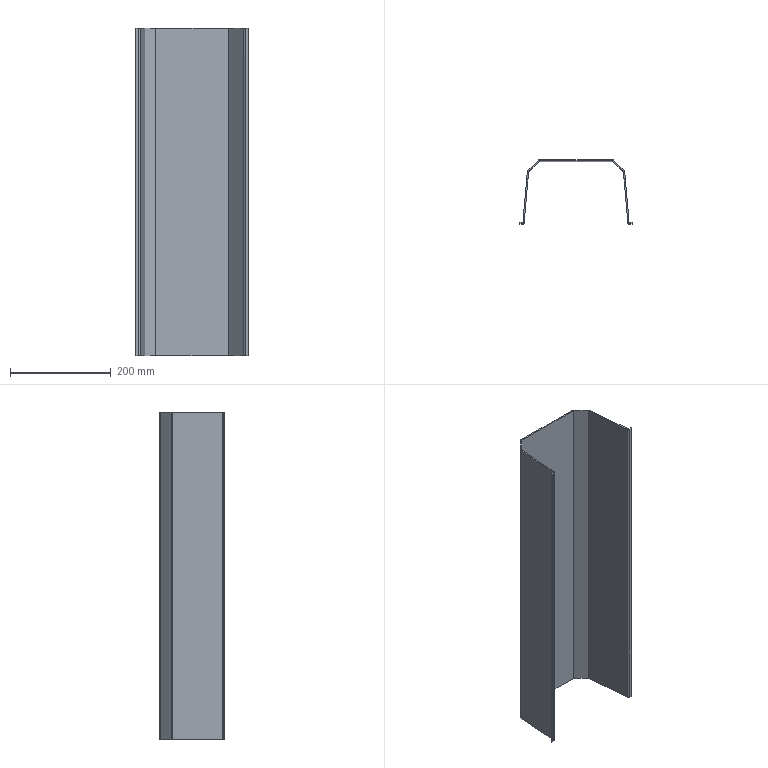Part | STEP file | 51E-01222JG10 | 1 solid | 56 faces | box 225 x 127 x 650 mm | volume 696230 mm3 | plane 40 | cylinder 16 | commonest cylinder face diameters 2 x6 7 x6 2.5 x4
STEP:
#1=CARTESIAN_POINT('',(-106.207,0.,325.));
#2=VERTEX_POINT('',#1);
#3=CARTESIAN_POINT('',(-106.207,2.5,325.));
#4=VERTEX_POINT('',#3);
#5=CARTESIAN_POINT('',(-106.207,1.25,325.));
#6=DIRECTION('',(0.,1.,0.));
#7=VECTOR('',#6,1.);
#8=LINE('',#5,#7);
#9=EDGE_CURVE('',#2,#4,#8,.T.);
#10=ORIENTED_EDGE('',*,*,#9,.F.);
#11=CARTESIAN_POINT('',(-102.72,3.195,325.));
#12=VERTEX_POINT('',#11);
#13=CARTESIAN_POINT('',(-102.72,3.195,325.));
#14=CARTESIAN_POINT('',(-102.752,2.83,325.));
#15=CARTESIAN_POINT('',(-102.832,2.469,325.));
#16=CARTESIAN_POINT('',(-102.959,2.12,325.));
#17=CARTESIAN_POINT('',(-103.301,1.465,325.));
#18=CARTESIAN_POINT('',(-103.8,0.9191,325.));
#19=CARTESIAN_POINT('',(-104.084,0.6808,325.));
#20=CARTESIAN_POINT('',(-104.656,0.3172,325.));
#21=CARTESIAN_POINT('',(-105.296,0.09984,325.));
#22=CARTESIAN_POINT('',(-105.597,0.03328,325.));
#23=CARTESIAN_POINT('',(-105.902,0.,325.));
#24=CARTESIAN_POINT('',(-106.207,0.,325.));
#25=B_SPLINE_CURVE_WITH_KNOTS('',5,(#13,#14,#15,#16,#17,#18,#19,#20,#21,#22,#23,#24),.UNSPECIFIED.,.F.,.U.,(6,3,3,6),(0.,2.592,5.185,7.343),.UNSPECIFIED.);
#26=EDGE_CURVE('',#12,#2,#25,.T.);
#27=ORIENTED_EDGE('',*,*,#26,.F.);
#28=CARTESIAN_POINT('',(-105.211,3.413,325.));
#29=VERTEX_POINT('',#28);
#30=CARTESIAN_POINT('',(-103.966,3.304,325.));
#31=DIRECTION('',(0.9962,-0.08716,0.));
#32=VECTOR('',#31,1.);
#33=LINE('',#30,#32);
#34=EDGE_CURVE('',#29,#12,#33,.T.);
#35=ORIENTED_EDGE('',*,*,#34,.F.);
#36=CARTESIAN_POINT('',(-105.211,3.413,325.));
#37=CARTESIAN_POINT('',(-105.22,3.315,325.));
#38=CARTESIAN_POINT('',(-105.24,3.219,325.));
#39=CARTESIAN_POINT('',(-105.272,3.125,325.));
#40=CARTESIAN_POINT('',(-105.359,2.948,325.));
#41=CARTESIAN_POINT('',(-105.486,2.797,325.));
#42=CARTESIAN_POINT('',(-105.559,2.729,325.));
#43=CARTESIAN_POINT('',(-105.719,2.614,325.));
#44=CARTESIAN_POINT('',(-105.902,2.54,325.));
#45=CARTESIAN_POINT('',(-105.998,2.515,325.));
#46=CARTESIAN_POINT('',(-106.098,2.501,325.));
#47=CARTESIAN_POINT('',(-106.199,2.5,325.));
#48=CARTESIAN_POINT('',(-106.202,2.5,325.));
#49=CARTESIAN_POINT('',(-106.204,2.5,325.));
#50=CARTESIAN_POINT('',(-106.207,2.5,325.));
#51=B_SPLINE_CURVE_WITH_KNOTS('',5,(#36,#37,#38,#39,#40,#41,#42,#43,#44,#45,#46,#47,#48,#49,#50),.UNSPECIFIED.,.F.,.U.,(6,3,3,3,6),(0.,0.6928,1.386,2.078,2.098),.UNSPECIFIED.);
#52=EDGE_CURVE('',#29,#4,#51,.T.);
#53=ORIENTED_EDGE('',*,*,#52,.T.);
#54=EDGE_LOOP('',(#10,#27,#35,#53));
#55=FACE_OUTER_BOUND('',#54,.T.);
#56=CARTESIAN_POINT('',(-106.207,0.,325.));
#57=DIRECTION('',(0.,0.,1.));
#58=DIRECTION('',(1.,0.,0.));
#59=AXIS2_PLACEMENT_3D('',#56,#57,#58);
#60=PLANE('',#59);
#61=ADVANCED_FACE('',(#55),#60,.T.);
#62=CARTESIAN_POINT('',(-111.25,2.5,325.));
#63=VERTEX_POINT('',#62);
#64=CARTESIAN_POINT('',(-112.5,1.25,325.));
#65=VERTEX_POINT('',#64);
#66=CARTESIAN_POINT('',(-111.25,1.25,325.));
#67=DIRECTION('',(0.,0.,1.));
#68=AXIS2_PLACEMENT_3D('',#66,#67,$);
#69=CIRCLE('',#68,1.25);
#70=EDGE_CURVE('',#63,#65,#69,.T.);
#71=ORIENTED_EDGE('',*,*,#70,.T.);
#72=CARTESIAN_POINT('',(-111.25,0.,325.));
#73=VERTEX_POINT('',#72);
#74=CARTESIAN_POINT('',(-111.25,1.25,325.));
#75=DIRECTION('',(0.,0.,1.));
#76=AXIS2_PLACEMENT_3D('',#74,#75,$);
#77=CIRCLE('',#76,1.25);
#78=EDGE_CURVE('',#65,#73,#77,.T.);
#79=ORIENTED_EDGE('',*,*,#78,.T.);
#80=CARTESIAN_POINT('',(-108.729,0.,325.));
#81=DIRECTION('',(-1.,0.,0.));
#82=VECTOR('',#81,1.);
#83=LINE('',#80,#82);
#84=EDGE_CURVE('',#2,#73,#83,.T.);
#85=ORIENTED_EDGE('',*,*,#84,.F.);
#86=ORIENTED_EDGE('',*,*,#9,.T.);
#87=CARTESIAN_POINT('',(-108.729,2.5,325.));
#88=DIRECTION('',(-1.,0.,0.));
#89=VECTOR('',#88,1.);
#90=LINE('',#87,#89);
#91=EDGE_CURVE('',#4,#63,#90,.T.);
#92=ORIENTED_EDGE('',*,*,#91,.T.);
#93=EDGE_LOOP('',(#71,#79,#85,#86,#92));
#94=FACE_OUTER_BOUND('',#93,.T.);
#95=CARTESIAN_POINT('',(-105.211,3.413,325.));
#96=DIRECTION('',(0.,0.,1.));
#97=DIRECTION('',(1.,0.,0.));
#98=AXIS2_PLACEMENT_3D('',#95,#96,#97);
#99=PLANE('',#98);
#100=ADVANCED_FACE('',(#94),#99,.T.);
#101=CARTESIAN_POINT('',(-102.72,3.195,-325.));
#102=VERTEX_POINT('',#101);
#103=CARTESIAN_POINT('',(-106.207,0.,-325.));
#104=VERTEX_POINT('',#103);
#105=CARTESIAN_POINT('',(-106.207,3.5,-325.));
#106=DIRECTION('',(0.,0.,-1.));
#107=AXIS2_PLACEMENT_3D('',#105,#106,$);
#108=CIRCLE('',#107,3.5);
#109=EDGE_CURVE('',#102,#104,#108,.T.);
#110=ORIENTED_EDGE('',*,*,#109,.F.);
#111=CARTESIAN_POINT('',(-102.72,3.195,325.));
#112=DIRECTION('',(0.,0.,-1.));
#113=VECTOR('',#112,1.);
#114=LINE('',#111,#113);
#115=EDGE_CURVE('',#12,#102,#114,.T.);
#116=ORIENTED_EDGE('',*,*,#115,.F.);
#117=ORIENTED_EDGE('',*,*,#26,.T.);
#118=CARTESIAN_POINT('',(-106.207,0.,325.));
#119=DIRECTION('',(0.,0.,-1.));
#120=VECTOR('',#119,1.);
#121=LINE('',#118,#120);
#122=EDGE_CURVE('',#2,#104,#121,.T.);
#123=ORIENTED_EDGE('',*,*,#122,.T.);
#124=EDGE_LOOP('',(#110,#116,#117,#123));
#125=FACE_OUTER_BOUND('',#124,.T.);
#126=CARTESIAN_POINT('',(-106.207,3.5,325.));
#127=DIRECTION('',(0.,0.,-1.));
#128=DIRECTION('',(1.,0.,0.));
#129=AXIS2_PLACEMENT_3D('',#126,#127,#128);
#130=CYLINDRICAL_SURFACE('',#129,3.5);
#131=ADVANCED_FACE('',(#125),#130,.T.);
#132=CARTESIAN_POINT('',(-94.02,102.637,325.));
#133=VERTEX_POINT('',#132);
#134=CARTESIAN_POINT('',(-98.37,52.916,325.));
#135=DIRECTION('',(-0.08716,-0.9962,0.));
#136=VECTOR('',#135,1.);
#137=LINE('',#134,#136);
#138=EDGE_CURVE('',#133,#12,#137,.T.);
#139=ORIENTED_EDGE('',*,*,#138,.F.);
#140=CARTESIAN_POINT('',(-96.511,102.855,325.));
#141=VERTEX_POINT('',#140);
#142=CARTESIAN_POINT('',(-95.266,102.746,325.));
#143=DIRECTION('',(-0.9962,0.08716,0.));
#144=VECTOR('',#143,1.);
#145=LINE('',#142,#144);
#146=EDGE_CURVE('',#133,#141,#145,.T.);
#147=ORIENTED_EDGE('',*,*,#146,.T.);
#148=CARTESIAN_POINT('',(-100.861,53.134,325.));
#149=DIRECTION('',(-0.08716,-0.9962,0.));
#150=VECTOR('',#149,1.);
#151=LINE('',#148,#150);
#152=EDGE_CURVE('',#141,#29,#151,.T.);
#153=ORIENTED_EDGE('',*,*,#152,.T.);
#154=ORIENTED_EDGE('',*,*,#34,.T.);
#155=EDGE_LOOP('',(#139,#147,#153,#154));
#156=FACE_OUTER_BOUND('',#155,.T.);
#157=CARTESIAN_POINT('',(-95.499,105.025,325.));
#158=DIRECTION('',(0.,0.,1.));
#159=DIRECTION('',(1.,0.,0.));
#160=AXIS2_PLACEMENT_3D('',#157,#158,#159);
#161=PLANE('',#160);
#162=ADVANCED_FACE('',(#156),#161,.T.);
#163=CARTESIAN_POINT('',(-105.211,3.413,-325.));
#164=VERTEX_POINT('',#163);
#165=CARTESIAN_POINT('',(-106.207,2.5,-325.));
#166=VERTEX_POINT('',#165);
#167=CARTESIAN_POINT('',(-106.207,3.5,-325.));
#168=DIRECTION('',(0.,0.,-1.));
#169=AXIS2_PLACEMENT_3D('',#167,#168,$);
#170=CIRCLE('',#169,1.);
#171=EDGE_CURVE('',#164,#166,#170,.T.);
#172=ORIENTED_EDGE('',*,*,#171,.T.);
#173=CARTESIAN_POINT('',(-106.207,2.5,325.));
#174=DIRECTION('',(0.,0.,-1.));
#175=VECTOR('',#174,1.);
#176=LINE('',#173,#175);
#177=EDGE_CURVE('',#4,#166,#176,.T.);
#178=ORIENTED_EDGE('',*,*,#177,.F.);
#179=ORIENTED_EDGE('',*,*,#52,.F.);
#180=CARTESIAN_POINT('',(-105.211,3.413,325.));
#181=DIRECTION('',(0.,0.,-1.));
#182=VECTOR('',#181,1.);
#183=LINE('',#180,#182);
#184=EDGE_CURVE('',#29,#164,#183,.T.);
#185=ORIENTED_EDGE('',*,*,#184,.T.);
#186=EDGE_LOOP('',(#172,#178,#179,#185));
#187=FACE_OUTER_BOUND('',#186,.T.);
#188=CARTESIAN_POINT('',(-106.207,3.5,325.));
#189=DIRECTION('',(0.,0.,-1.));
#190=DIRECTION('',(1.,0.,0.));
#191=AXIS2_PLACEMENT_3D('',#188,#189,#190);
#192=CYLINDRICAL_SURFACE('',#191,1.);
#193=ADVANCED_FACE('',(#187),#192,.F.);
#194=CARTESIAN_POINT('',(-112.5,1.25,-325.));
#195=VERTEX_POINT('',#194);
#196=CARTESIAN_POINT('',(-112.5,1.25,325.));
#197=DIRECTION('',(0.,0.,1.));
#198=VECTOR('',#197,1.);
#199=LINE('',#196,#198);
#200=EDGE_CURVE('',#65,#195,#199,.F.);
#201=ORIENTED_EDGE('',*,*,#200,.F.);
#202=ORIENTED_EDGE('',*,*,#70,.F.);
#203=CARTESIAN_POINT('',(-111.25,2.5,-325.));
#204=VERTEX_POINT('',#203);
#205=CARTESIAN_POINT('',(-111.25,2.5,325.));
#206=DIRECTION('',(0.,0.,1.));
#207=VECTOR('',#206,1.);
#208=LINE('',#205,#207);
#209=EDGE_CURVE('',#204,#63,#208,.T.);
#210=ORIENTED_EDGE('',*,*,#209,.F.);
#211=CARTESIAN_POINT('',(-111.25,1.25,-325.));
#212=DIRECTION('',(0.,0.,1.));
#213=AXIS2_PLACEMENT_3D('',#211,#212,$);
#214=CIRCLE('',#213,1.25);
#215=EDGE_CURVE('',#195,#204,#214,.F.);
#216=ORIENTED_EDGE('',*,*,#215,.F.);
#217=EDGE_LOOP('',(#201,#202,#210,#216));
#218=FACE_OUTER_BOUND('',#217,.T.);
#219=CARTESIAN_POINT('',(-111.25,1.25,325.));
#220=DIRECTION('',(0.,0.,1.));
#221=DIRECTION('',(1.,0.,0.));
#222=AXIS2_PLACEMENT_3D('',#219,#220,#221);
#223=CYLINDRICAL_SURFACE('',#222,1.25);
#224=ADVANCED_FACE('',(#218),#223,.T.);
#225=ORIENTED_EDGE('',*,*,#78,.F.);
#226=ORIENTED_EDGE('',*,*,#200,.T.);
#227=CARTESIAN_POINT('',(-111.25,0.,-325.));
#228=VERTEX_POINT('',#227);
#229=CARTESIAN_POINT('',(-111.25,1.25,-325.));
#230=DIRECTION('',(0.,0.,-1.));
#231=AXIS2_PLACEMENT_3D('',#229,#230,$);
#232=CIRCLE('',#231,1.25);
#233=EDGE_CURVE('',#228,#195,#232,.T.);
#234=ORIENTED_EDGE('',*,*,#233,.F.);
#235=CARTESIAN_POINT('',(-111.25,0.,325.));
#236=DIRECTION('',(0.,0.,-1.));
#237=VECTOR('',#236,1.);
#238=LINE('',#235,#237);
#239=EDGE_CURVE('',#73,#228,#238,.T.);
#240=ORIENTED_EDGE('',*,*,#239,.F.);
#241=EDGE_LOOP('',(#225,#226,#234,#240));
#242=FACE_OUTER_BOUND('',#241,.T.);
#243=CARTESIAN_POINT('',(-111.25,1.25,325.));
#244=DIRECTION('',(0.,0.,-1.));
#245=DIRECTION('',(1.,0.,0.));
#246=AXIS2_PLACEMENT_3D('',#243,#244,#245);
#247=CYLINDRICAL_SURFACE('',#246,1.25);
#248=ADVANCED_FACE('',(#242),#247,.T.);
#249=ORIENTED_EDGE('',*,*,#84,.T.);
#250=ORIENTED_EDGE('',*,*,#239,.T.);
#251=CARTESIAN_POINT('',(-108.729,0.,-325.));
#252=DIRECTION('',(-1.,0.,0.));
#253=VECTOR('',#252,1.);
#254=LINE('',#251,#253);
#255=EDGE_CURVE('',#104,#228,#254,.T.);
#256=ORIENTED_EDGE('',*,*,#255,.F.);
#257=ORIENTED_EDGE('',*,*,#122,.F.);
#258=EDGE_LOOP('',(#249,#250,#256,#257));
#259=FACE_OUTER_BOUND('',#258,.T.);
#260=CARTESIAN_POINT('',(-112.5,0.,325.));
#261=DIRECTION('',(0.,-1.,0.));
#262=DIRECTION('',(0.,0.,-1.));
#263=AXIS2_PLACEMENT_3D('',#260,#261,#262);
#264=PLANE('',#263);
#265=ADVANCED_FACE('',(#259),#264,.T.);
#266=CARTESIAN_POINT('',(-108.729,2.5,-325.));
#267=DIRECTION('',(-1.,0.,0.));
#268=VECTOR('',#267,1.);
#269=LINE('',#266,#268);
#270=EDGE_CURVE('',#166,#204,#269,.T.);
#271=ORIENTED_EDGE('',*,*,#270,.T.);
#272=ORIENTED_EDGE('',*,*,#209,.T.);
#273=ORIENTED_EDGE('',*,*,#91,.F.);
#274=ORIENTED_EDGE('',*,*,#177,.T.);
#275=EDGE_LOOP('',(#271,#272,#273,#274));
#276=FACE_OUTER_BOUND('',#275,.T.);
#277=CARTESIAN_POINT('',(-112.5,2.5,325.));
#278=DIRECTION('',(0.,-1.,0.));
#279=DIRECTION('',(0.,0.,-1.));
#280=AXIS2_PLACEMENT_3D('',#277,#278,#279);
#281=PLANE('',#280);
#282=ADVANCED_FACE('',(#276),#281,.F.);
#283=CARTESIAN_POINT('',(-103.966,3.304,-325.));
#284=DIRECTION('',(-0.9962,0.08716,0.));
#285=VECTOR('',#284,1.);
#286=LINE('',#283,#285);
#287=EDGE_CURVE('',#102,#164,#286,.T.);
#288=ORIENTED_EDGE('',*,*,#287,.F.);
#289=ORIENTED_EDGE('',*,*,#109,.T.);
#290=CARTESIAN_POINT('',(-106.207,1.25,-325.));
#291=DIRECTION('',(0.,-1.,0.));
#292=VECTOR('',#291,1.);
#293=LINE('',#290,#292);
#294=EDGE_CURVE('',#166,#104,#293,.T.);
#295=ORIENTED_EDGE('',*,*,#294,.F.);
#296=ORIENTED_EDGE('',*,*,#171,.F.);
#297=EDGE_LOOP('',(#288,#289,#295,#296));
#298=FACE_OUTER_BOUND('',#297,.T.);
#299=CARTESIAN_POINT('',(-102.72,3.195,-325.));
#300=DIRECTION('',(0.,0.,-1.));
#301=DIRECTION('',(-1.,0.,0.));
#302=AXIS2_PLACEMENT_3D('',#299,#300,#301);
#303=PLANE('',#302);
#304=ADVANCED_FACE('',(#298),#303,.T.);
#305=CARTESIAN_POINT('',(-94.02,102.637,-325.));
#306=VERTEX_POINT('',#305);
#307=CARTESIAN_POINT('',(-98.37,52.916,-325.));
#308=DIRECTION('',(-0.08716,-0.9962,0.));
#309=VECTOR('',#308,1.);
#310=LINE('',#307,#309);
#311=EDGE_CURVE('',#306,#102,#310,.T.);
#312=ORIENTED_EDGE('',*,*,#311,.F.);
#313=CARTESIAN_POINT('',(-94.02,102.637,0.));
#314=DIRECTION('',(0.,0.,-1.));
#315=VECTOR('',#314,1.);
#316=LINE('',#313,#315);
#317=EDGE_CURVE('',#133,#306,#316,.T.);
#318=ORIENTED_EDGE('',*,*,#317,.F.);
#319=ORIENTED_EDGE('',*,*,#138,.T.);
#320=ORIENTED_EDGE('',*,*,#115,.T.);
#321=EDGE_LOOP('',(#312,#318,#319,#320));
#322=FACE_OUTER_BOUND('',#321,.T.);
#323=CARTESIAN_POINT('',(-103.,0.,325.));
#324=DIRECTION('',(0.9962,-0.08716,0.));
#325=DIRECTION('',(0.08716,0.9962,0.));
#326=AXIS2_PLACEMENT_3D('',#323,#324,#325);
#327=PLANE('',#326);
#328=ADVANCED_FACE('',(#322),#327,.T.);
#329=ORIENTED_EDGE('',*,*,#146,.F.);
#330=CARTESIAN_POINT('',(-93.731,103.257,325.));
#331=VERTEX_POINT('',#330);
#332=CARTESIAN_POINT('',(-93.024,102.55,325.));
#333=DIRECTION('',(0.,0.,1.));
#334=AXIS2_PLACEMENT_3D('',#332,#333,$);
#335=CIRCLE('',#334,1.);
#336=EDGE_CURVE('',#331,#133,#335,.T.);
#337=ORIENTED_EDGE('',*,*,#336,.F.);
#338=CARTESIAN_POINT('',(-95.499,105.025,325.));
#339=VERTEX_POINT('',#338);
#340=CARTESIAN_POINT('',(-94.615,104.141,325.));
#341=DIRECTION('',(0.7071,-0.7071,0.));
#342=VECTOR('',#341,1.);
#343=LINE('',#340,#342);
#344=EDGE_CURVE('',#339,#331,#343,.T.);
#345=ORIENTED_EDGE('',*,*,#344,.F.);
#346=CARTESIAN_POINT('',(-93.024,102.55,325.));
#347=DIRECTION('',(0.,0.,1.));
#348=AXIS2_PLACEMENT_3D('',#346,#347,$);
#349=CIRCLE('',#348,3.5);
#350=EDGE_CURVE('',#339,#141,#349,.T.);
#351=ORIENTED_EDGE('',*,*,#350,.T.);
#352=EDGE_LOOP('',(#329,#337,#345,#351));
#353=FACE_OUTER_BOUND('',#352,.T.);
#354=CARTESIAN_POINT('',(-94.02,102.637,325.));
#355=DIRECTION('',(0.,0.,1.));
#356=DIRECTION('',(1.,0.,0.));
#357=AXIS2_PLACEMENT_3D('',#354,#355,#356);
#358=PLANE('',#357);
#359=ADVANCED_FACE('',(#353),#358,.T.);
#360=CARTESIAN_POINT('',(-96.511,102.855,-325.));
#361=VERTEX_POINT('',#360);
#362=CARTESIAN_POINT('',(-100.861,53.134,-325.));
#363=DIRECTION('',(-0.08716,-0.9962,0.));
#364=VECTOR('',#363,1.);
#365=LINE('',#362,#364);
#366=EDGE_CURVE('',#361,#164,#365,.T.);
#367=ORIENTED_EDGE('',*,*,#366,.T.);
#368=ORIENTED_EDGE('',*,*,#184,.F.);
#369=ORIENTED_EDGE('',*,*,#152,.F.);
#370=CARTESIAN_POINT('',(-96.511,102.855,0.));
#371=DIRECTION('',(0.,0.,-1.));
#372=VECTOR('',#371,1.);
#373=LINE('',#370,#372);
#374=EDGE_CURVE('',#141,#361,#373,.T.);
#375=ORIENTED_EDGE('',*,*,#374,.T.);
#376=EDGE_LOOP('',(#367,#368,#369,#375));
#377=FACE_OUTER_BOUND('',#376,.T.);
#378=CARTESIAN_POINT('',(-105.49,0.2179,325.));
#379=DIRECTION('',(0.9962,-0.08716,0.));
#380=DIRECTION('',(0.08716,0.9962,0.));
#381=AXIS2_PLACEMENT_3D('',#378,#379,#380);
#382=PLANE('',#381);
#383=ADVANCED_FACE('',(#377),#382,.F.);
#384=ORIENTED_EDGE('',*,*,#255,.T.);
#385=ORIENTED_EDGE('',*,*,#233,.T.);
#386=ORIENTED_EDGE('',*,*,#215,.T.);
#387=ORIENTED_EDGE('',*,*,#270,.F.);
#388=ORIENTED_EDGE('',*,*,#294,.T.);
#389=EDGE_LOOP('',(#384,#385,#386,#387,#388));
#390=FACE_OUTER_BOUND('',#389,.T.);
#391=CARTESIAN_POINT('',(-106.207,3.5,-325.));
#392=DIRECTION('',(0.,0.,-1.));
#393=DIRECTION('',(-1.,0.,0.));
#394=AXIS2_PLACEMENT_3D('',#391,#392,#393);
#395=PLANE('',#394);
#396=ADVANCED_FACE('',(#390),#395,.T.);
#397=ORIENTED_EDGE('',*,*,#311,.T.);
#398=ORIENTED_EDGE('',*,*,#287,.T.);
#399=ORIENTED_EDGE('',*,*,#366,.F.);
#400=CARTESIAN_POINT('',(-95.266,102.746,-325.));
#401=DIRECTION('',(0.9962,-0.08716,0.));
#402=VECTOR('',#401,1.);
#403=LINE('',#400,#402);
#404=EDGE_CURVE('',#361,#306,#403,.T.);
#405=ORIENTED_EDGE('',*,*,#404,.T.);
#406=EDGE_LOOP('',(#397,#398,#399,#405));
#407=FACE_OUTER_BOUND('',#406,.T.);
#408=CARTESIAN_POINT('',(-106.207,2.5,-325.));
#409=DIRECTION('',(0.,0.,-1.));
#410=DIRECTION('',(-1.,0.,0.));
#411=AXIS2_PLACEMENT_3D('',#408,#409,#410);
#412=PLANE('',#411);
#413=ADVANCED_FACE('',(#407),#412,.T.);
#414=CARTESIAN_POINT('',(-93.731,103.257,-325.));
#415=VERTEX_POINT('',#414);
#416=CARTESIAN_POINT('',(-93.024,102.55,-325.));
#417=DIRECTION('',(0.,0.,-1.));
#418=AXIS2_PLACEMENT_3D('',#416,#417,$);
#419=CIRCLE('',#418,1.);
#420=EDGE_CURVE('',#415,#306,#419,.F.);
#421=ORIENTED_EDGE('',*,*,#420,.F.);
#422=CARTESIAN_POINT('',(-93.731,103.257,325.));
#423=DIRECTION('',(0.,0.,-1.));
#424=VECTOR('',#423,1.);
#425=LINE('',#422,#424);
#426=EDGE_CURVE('',#331,#415,#425,.T.);
#427=ORIENTED_EDGE('',*,*,#426,.F.);
#428=ORIENTED_EDGE('',*,*,#336,.T.);
#429=ORIENTED_EDGE('',*,*,#317,.T.);
#430=EDGE_LOOP('',(#421,#427,#428,#429));
#431=FACE_OUTER_BOUND('',#430,.T.);
#432=CARTESIAN_POINT('',(-93.024,102.55,325.));
#433=DIRECTION('',(0.,0.,-1.));
#434=DIRECTION('',(-1.,0.,0.));
#435=AXIS2_PLACEMENT_3D('',#432,#433,#434);
#436=CYLINDRICAL_SURFACE('',#435,1.);
#437=ADVANCED_FACE('',(#431),#436,.F.);
#438=CARTESIAN_POINT('',(-72.782,124.207,325.));
#439=VERTEX_POINT('',#438);
#440=CARTESIAN_POINT('',(-83.256,113.732,325.));
#441=DIRECTION('',(-0.7071,-0.7071,0.));
#442=VECTOR('',#441,1.);
#443=LINE('',#440,#442);
#444=EDGE_CURVE('',#439,#331,#443,.T.);
#445=ORIENTED_EDGE('',*,*,#444,.F.);
#446=CARTESIAN_POINT('',(-74.549,125.975,325.));
#447=VERTEX_POINT('',#446);
#448=CARTESIAN_POINT('',(-73.665,125.091,325.));
#449=DIRECTION('',(-0.7071,0.7071,0.));
#450=VECTOR('',#449,1.);
#451=LINE('',#448,#450);
#452=EDGE_CURVE('',#439,#447,#451,.T.);
#453=ORIENTED_EDGE('',*,*,#452,.T.);
#454=CARTESIAN_POINT('',(-85.024,115.5,325.));
#455=DIRECTION('',(-0.7071,-0.7071,0.));
#456=VECTOR('',#455,1.);
#457=LINE('',#454,#456);
#458=EDGE_CURVE('',#447,#339,#457,.T.);
#459=ORIENTED_EDGE('',*,*,#458,.T.);
#460=ORIENTED_EDGE('',*,*,#344,.T.);
#461=EDGE_LOOP('',(#445,#453,#459,#460));
#462=FACE_OUTER_BOUND('',#461,.T.);
#463=CARTESIAN_POINT('',(-72.074,127.,325.));
#464=DIRECTION('',(0.,0.,1.));
#465=DIRECTION('',(1.,0.,0.));
#466=AXIS2_PLACEMENT_3D('',#463,#464,#465);
#467=PLANE('',#466);
#468=ADVANCED_FACE('',(#462),#467,.T.);
#469=CARTESIAN_POINT('',(-95.499,105.025,-325.));
#470=VERTEX_POINT('',#469);
#471=CARTESIAN_POINT('',(-93.024,102.55,-325.));
#472=DIRECTION('',(0.,0.,-1.));
#473=AXIS2_PLACEMENT_3D('',#471,#472,$);
#474=CIRCLE('',#473,3.5);
#475=EDGE_CURVE('',#470,#361,#474,.F.);
#476=ORIENTED_EDGE('',*,*,#475,.T.);
#477=ORIENTED_EDGE('',*,*,#374,.F.);
#478=ORIENTED_EDGE('',*,*,#350,.F.);
#479=CARTESIAN_POINT('',(-95.499,105.025,325.));
#480=DIRECTION('',(0.,0.,-1.));
#481=VECTOR('',#480,1.);
#482=LINE('',#479,#481);
#483=EDGE_CURVE('',#339,#470,#482,.T.);
#484=ORIENTED_EDGE('',*,*,#483,.T.);
#485=EDGE_LOOP('',(#476,#477,#478,#484));
#486=FACE_OUTER_BOUND('',#485,.T.);
#487=CARTESIAN_POINT('',(-93.024,102.55,325.));
#488=DIRECTION('',(0.,0.,-1.));
#489=DIRECTION('',(-1.,0.,0.));
#490=AXIS2_PLACEMENT_3D('',#487,#488,#489);
#491=CYLINDRICAL_SURFACE('',#490,3.5);
#492=ADVANCED_FACE('',(#486),#491,.T.);
#493=CARTESIAN_POINT('',(-94.615,104.141,-325.));
#494=DIRECTION('',(-0.7071,0.7071,0.));
#495=VECTOR('',#494,1.);
#496=LINE('',#493,#495);
#497=EDGE_CURVE('',#415,#470,#496,.T.);
#498=ORIENTED_EDGE('',*,*,#497,.F.);
#499=ORIENTED_EDGE('',*,*,#420,.T.);
#500=ORIENTED_EDGE('',*,*,#404,.F.);
#501=ORIENTED_EDGE('',*,*,#475,.F.);
#502=EDGE_LOOP('',(#498,#499,#500,#501));
#503=FACE_OUTER_BOUND('',#502,.T.);
#504=CARTESIAN_POINT('',(-93.731,103.257,-325.));
#505=DIRECTION('',(0.,0.,-1.));
#506=DIRECTION('',(-1.,0.,0.));
#507=AXIS2_PLACEMENT_3D('',#504,#505,#506);
#508=PLANE('',#507);
#509=ADVANCED_FACE('',(#503),#508,.T.);
#510=CARTESIAN_POINT('',(-72.782,124.207,-325.));
#511=VERTEX_POINT('',#510);
#512=CARTESIAN_POINT('',(-83.256,113.732,-325.));
#513=DIRECTION('',(-0.7071,-0.7071,0.));
#514=VECTOR('',#513,1.);
#515=LINE('',#512,#514);
#516=EDGE_CURVE('',#511,#415,#515,.T.);
#517=ORIENTED_EDGE('',*,*,#516,.F.);
#518=CARTESIAN_POINT('',(-72.782,124.207,0.));
#519=DIRECTION('',(0.,0.,-1.));
#520=VECTOR('',#519,1.);
#521=LINE('',#518,#520);
#522=EDGE_CURVE('',#439,#511,#521,.T.);
#523=ORIENTED_EDGE('',*,*,#522,.F.);
#524=ORIENTED_EDGE('',*,*,#444,.T.);
#525=ORIENTED_EDGE('',*,*,#426,.T.);
#526=EDGE_LOOP('',(#517,#523,#524,#525));
#527=FACE_OUTER_BOUND('',#526,.T.);
#528=CARTESIAN_POINT('',(-93.989,103.,325.));
#529=DIRECTION('',(0.7071,-0.7071,0.));
#530=DIRECTION('',(0.7071,0.7071,0.));
#531=AXIS2_PLACEMENT_3D('',#528,#529,#530);
#532=PLANE('',#531);
#533=ADVANCED_FACE('',(#527),#532,.T.);
#534=ORIENTED_EDGE('',*,*,#452,.F.);
#535=CARTESIAN_POINT('',(-72.074,124.5,325.));
#536=VERTEX_POINT('',#535);
#537=CARTESIAN_POINT('',(-72.074,123.5,325.));
#538=DIRECTION('',(0.,0.,1.));
#539=AXIS2_PLACEMENT_3D('',#537,#538,$);
#540=CIRCLE('',#539,1.);
#541=EDGE_CURVE('',#536,#439,#540,.T.);
#542=ORIENTED_EDGE('',*,*,#541,.F.);
#543=CARTESIAN_POINT('',(-72.074,127.,325.));
#544=VERTEX_POINT('',#543);
#545=CARTESIAN_POINT('',(-72.074,125.75,325.));
#546=DIRECTION('',(0.,-1.,0.));
#547=VECTOR('',#546,1.);
#548=LINE('',#545,#547);
#549=EDGE_CURVE('',#544,#536,#548,.T.);
#550=ORIENTED_EDGE('',*,*,#549,.F.);
#551=CARTESIAN_POINT('',(-72.074,123.5,325.));
#552=DIRECTION('',(0.,0.,1.));
#553=AXIS2_PLACEMENT_3D('',#551,#552,$);
#554=CIRCLE('',#553,3.5);
#555=EDGE_CURVE('',#544,#447,#554,.T.);
#556=ORIENTED_EDGE('',*,*,#555,.T.);
#557=EDGE_LOOP('',(#534,#542,#550,#556));
#558=FACE_OUTER_BOUND('',#557,.T.);
#559=CARTESIAN_POINT('',(-72.782,124.207,325.));
#560=DIRECTION('',(0.,0.,1.));
#561=DIRECTION('',(1.,0.,0.));
#562=AXIS2_PLACEMENT_3D('',#559,#560,#561);
#563=PLANE('',#562);
#564=ADVANCED_FACE('',(#558),#563,.T.);
#565=CARTESIAN_POINT('',(-74.549,125.975,-325.));
#566=VERTEX_POINT('',#565);
#567=CARTESIAN_POINT('',(-85.024,115.5,-325.));
#568=DIRECTION('',(-0.7071,-0.7071,0.));
#569=VECTOR('',#568,1.);
#570=LINE('',#567,#569);
#571=EDGE_CURVE('',#566,#470,#570,.T.);
#572=ORIENTED_EDGE('',*,*,#571,.T.);
#573=ORIENTED_EDGE('',*,*,#483,.F.);
#574=ORIENTED_EDGE('',*,*,#458,.F.);
#575=CARTESIAN_POINT('',(-74.549,125.975,0.));
#576=DIRECTION('',(0.,0.,-1.));
#577=VECTOR('',#576,1.);
#578=LINE('',#575,#577);
#579=EDGE_CURVE('',#447,#566,#578,.T.);
#580=ORIENTED_EDGE('',*,*,#579,.T.);
#581=EDGE_LOOP('',(#572,#573,#574,#580));
#582=FACE_OUTER_BOUND('',#581,.T.);
#583=CARTESIAN_POINT('',(-95.756,104.768,325.));
#584=DIRECTION('',(0.7071,-0.7071,0.));
#585=DIRECTION('',(0.7071,0.7071,0.));
#586=AXIS2_PLACEMENT_3D('',#583,#584,#585);
#587=PLANE('',#586);
#588=ADVANCED_FACE('',(#582),#587,.F.);
#589=ORIENTED_EDGE('',*,*,#516,.T.);
#590=ORIENTED_EDGE('',*,*,#497,.T.);
#591=ORIENTED_EDGE('',*,*,#571,.F.);
#592=CARTESIAN_POINT('',(-73.665,125.091,-325.));
#593=DIRECTION('',(0.7071,-0.7071,0.));
#594=VECTOR('',#593,1.);
#595=LINE('',#592,#594);
#596=EDGE_CURVE('',#566,#511,#595,.T.);
#597=ORIENTED_EDGE('',*,*,#596,.T.);
#598=EDGE_LOOP('',(#589,#590,#591,#597));
#599=FACE_OUTER_BOUND('',#598,.T.);
#600=CARTESIAN_POINT('',(-96.511,102.855,-325.));
#601=DIRECTION('',(0.,0.,-1.));
#602=DIRECTION('',(-1.,0.,0.));
#603=AXIS2_PLACEMENT_3D('',#600,#601,#602);
#604=PLANE('',#603);
#605=ADVANCED_FACE('',(#599),#604,.T.);
#606=CARTESIAN_POINT('',(-72.074,124.5,-325.));
#607=VERTEX_POINT('',#606);
#608=CARTESIAN_POINT('',(-72.074,123.5,-325.));
#609=DIRECTION('',(0.,0.,-1.));
#610=AXIS2_PLACEMENT_3D('',#608,#609,$);
#611=CIRCLE('',#610,1.);
#612=EDGE_CURVE('',#607,#511,#611,.F.);
#613=ORIENTED_EDGE('',*,*,#612,.F.);
#614=CARTESIAN_POINT('',(-72.074,124.5,325.));
#615=DIRECTION('',(0.,0.,-1.));
#616=VECTOR('',#615,1.);
#617=LINE('',#614,#616);
#618=EDGE_CURVE('',#536,#607,#617,.T.);
#619=ORIENTED_EDGE('',*,*,#618,.F.);
#620=ORIENTED_EDGE('',*,*,#541,.T.);
#621=ORIENTED_EDGE('',*,*,#522,.T.);
#622=EDGE_LOOP('',(#613,#619,#620,#621));
#623=FACE_OUTER_BOUND('',#622,.T.);
#624=CARTESIAN_POINT('',(-72.074,123.5,325.));
#625=DIRECTION('',(0.,0.,-1.));
#626=DIRECTION('',(-1.,0.,0.));
#627=AXIS2_PLACEMENT_3D('',#624,#625,#626);
#628=CYLINDRICAL_SURFACE('',#627,1.);
#629=ADVANCED_FACE('',(#623),#628,.F.);
#630=CARTESIAN_POINT('',(72.074,124.5,325.));
#631=VERTEX_POINT('',#630);
#632=CARTESIAN_POINT('',(0.,124.5,325.));
#633=DIRECTION('',(-1.,0.,0.));
#634=VECTOR('',#633,1.);
#635=LINE('',#632,#634);
#636=EDGE_CURVE('',#631,#536,#635,.T.);
#637=ORIENTED_EDGE('',*,*,#636,.F.);
#638=CARTESIAN_POINT('',(72.074,127.,325.));
#639=VERTEX_POINT('',#638);
#640=CARTESIAN_POINT('',(72.074,125.75,325.));
#641=DIRECTION('',(0.,1.,0.));
#642=VECTOR('',#641,1.);
#643=LINE('',#640,#642);
#644=EDGE_CURVE('',#631,#639,#643,.T.);
#645=ORIENTED_EDGE('',*,*,#644,.T.);
#646=CARTESIAN_POINT('',(0.,127.,325.));
#647=DIRECTION('',(-1.,0.,0.));
#648=VECTOR('',#647,1.);
#649=LINE('',#646,#648);
#650=EDGE_CURVE('',#639,#544,#649,.T.);
#651=ORIENTED_EDGE('',*,*,#650,.T.);
#652=ORIENTED_EDGE('',*,*,#549,.T.);
#653=EDGE_LOOP('',(#637,#645,#651,#652));
#654=FACE_OUTER_BOUND('',#653,.T.);
#655=CARTESIAN_POINT('',(74.549,125.975,325.));
#656=DIRECTION('',(0.,0.,1.));
#657=DIRECTION('',(1.,0.,0.));
#658=AXIS2_PLACEMENT_3D('',#655,#656,#657);
#659=PLANE('',#658);
#660=ADVANCED_FACE('',(#654),#659,.T.);
#661=CARTESIAN_POINT('',(-72.074,127.,-325.));
#662=VERTEX_POINT('',#661);
#663=CARTESIAN_POINT('',(-72.074,123.5,-325.));
#664=DIRECTION('',(0.,0.,-1.));
#665=AXIS2_PLACEMENT_3D('',#663,#664,$);
#666=CIRCLE('',#665,3.5);
#667=EDGE_CURVE('',#662,#566,#666,.F.);
#668=ORIENTED_EDGE('',*,*,#667,.T.);
#669=ORIENTED_EDGE('',*,*,#579,.F.);
#670=ORIENTED_EDGE('',*,*,#555,.F.);
#671=CARTESIAN_POINT('',(-72.074,127.,325.));
#672=DIRECTION('',(0.,0.,-1.));
#673=VECTOR('',#672,1.);
#674=LINE('',#671,#673);
#675=EDGE_CURVE('',#544,#662,#674,.T.);
#676=ORIENTED_EDGE('',*,*,#675,.T.);
#677=EDGE_LOOP('',(#668,#669,#670,#676));
#678=FACE_OUTER_BOUND('',#677,.T.);
#679=CARTESIAN_POINT('',(-72.074,123.5,325.));
#680=DIRECTION('',(0.,0.,-1.));
#681=DIRECTION('',(-1.,0.,0.));
#682=AXIS2_PLACEMENT_3D('',#679,#680,#681);
#683=CYLINDRICAL_SURFACE('',#682,3.5);
#684=ADVANCED_FACE('',(#678),#683,.T.);
#685=CARTESIAN_POINT('',(-72.074,125.75,-325.));
#686=DIRECTION('',(0.,1.,0.));
#687=VECTOR('',#686,1.);
#688=LINE('',#685,#687);
#689=EDGE_CURVE('',#607,#662,#688,.T.);
#690=ORIENTED_EDGE('',*,*,#689,.F.);
#691=ORIENTED_EDGE('',*,*,#612,.T.);
#692=ORIENTED_EDGE('',*,*,#596,.F.);
#693=ORIENTED_EDGE('',*,*,#667,.F.);
#694=EDGE_LOOP('',(#690,#691,#692,#693));
#695=FACE_OUTER_BOUND('',#694,.T.);
#696=CARTESIAN_POINT('',(-72.074,124.5,-325.));
#697=DIRECTION('',(0.,0.,-1.));
#698=DIRECTION('',(-1.,0.,0.));
#699=AXIS2_PLACEMENT_3D('',#696,#697,#698);
#700=PLANE('',#699);
#701=ADVANCED_FACE('',(#695),#700,.T.);
#702=CARTESIAN_POINT('',(72.074,124.5,-325.));
#703=VERTEX_POINT('',#702);
#704=CARTESIAN_POINT('',(0.,124.5,-325.));
#705=DIRECTION('',(-1.,0.,0.));
#706=VECTOR('',#705,1.);
#707=LINE('',#704,#706);
#708=EDGE_CURVE('',#703,#607,#707,.T.);
#709=ORIENTED_EDGE('',*,*,#708,.F.);
#710=CARTESIAN_POINT('',(72.074,124.5,0.));
#711=DIRECTION('',(0.,0.,-1.));
#712=VECTOR('',#711,1.);
#713=LINE('',#710,#712);
#714=EDGE_CURVE('',#631,#703,#713,.T.);
#715=ORIENTED_EDGE('',*,*,#714,.F.);
#716=ORIENTED_EDGE('',*,*,#636,.T.);
#717=ORIENTED_EDGE('',*,*,#618,.T.);
#718=EDGE_LOOP('',(#709,#715,#716,#717));
#719=FACE_OUTER_BOUND('',#718,.T.);
#720=CARTESIAN_POINT('',(-72.489,124.5,325.));
#721=DIRECTION('',(0.,-1.,0.));
#722=DIRECTION('',(0.,0.,-1.));
#723=AXIS2_PLACEMENT_3D('',#720,#721,#722);
#724=PLANE('',#723);
#725=ADVANCED_FACE('',(#719),#724,.T.);
#726=ORIENTED_EDGE('',*,*,#644,.F.);
#727=CARTESIAN_POINT('',(72.782,124.207,325.));
#728=VERTEX_POINT('',#727);
#729=CARTESIAN_POINT('',(72.074,123.5,325.));
#730=DIRECTION('',(0.,0.,1.));
#731=AXIS2_PLACEMENT_3D('',#729,#730,$);
#732=CIRCLE('',#731,1.);
#733=EDGE_CURVE('',#728,#631,#732,.T.);
#734=ORIENTED_EDGE('',*,*,#733,.F.);
#735=CARTESIAN_POINT('',(74.549,125.975,325.));
#736=VERTEX_POINT('',#735);
#737=CARTESIAN_POINT('',(73.665,125.091,325.));
#738=DIRECTION('',(-0.7071,-0.7071,0.));
#739=VECTOR('',#738,1.);
#740=LINE('',#737,#739);
#741=EDGE_CURVE('',#736,#728,#740,.T.);
#742=ORIENTED_EDGE('',*,*,#741,.F.);
#743=CARTESIAN_POINT('',(72.074,123.5,325.));
#744=DIRECTION('',(0.,0.,1.));
#745=AXIS2_PLACEMENT_3D('',#743,#744,$);
#746=CIRCLE('',#745,3.5);
#747=EDGE_CURVE('',#736,#639,#746,.T.);
#748=ORIENTED_EDGE('',*,*,#747,.T.);
#749=EDGE_LOOP('',(#726,#734,#742,#748));
#750=FACE_OUTER_BOUND('',#749,.T.);
#751=CARTESIAN_POINT('',(72.074,124.5,325.));
#752=DIRECTION('',(0.,0.,1.));
#753=DIRECTION('',(1.,0.,0.));
#754=AXIS2_PLACEMENT_3D('',#751,#752,#753);
#755=PLANE('',#754);
#756=ADVANCED_FACE('',(#750),#755,.T.);
#757=CARTESIAN_POINT('',(72.074,127.,-325.));
#758=VERTEX_POINT('',#757);
#759=CARTESIAN_POINT('',(0.,127.,-325.));
#760=DIRECTION('',(-1.,0.,0.));
#761=VECTOR('',#760,1.);
#762=LINE('',#759,#761);
#763=EDGE_CURVE('',#758,#662,#762,.T.);
#764=ORIENTED_EDGE('',*,*,#763,.T.);
#765=ORIENTED_EDGE('',*,*,#675,.F.);
#766=ORIENTED_EDGE('',*,*,#650,.F.);
#767=CARTESIAN_POINT('',(72.074,127.,0.));
#768=DIRECTION('',(0.,0.,-1.));
#769=VECTOR('',#768,1.);
#770=LINE('',#767,#769);
#771=EDGE_CURVE('',#639,#758,#770,.T.);
#772=ORIENTED_EDGE('',*,*,#771,.T.);
#773=EDGE_LOOP('',(#764,#765,#766,#772));
#774=FACE_OUTER_BOUND('',#773,.T.);
#775=CARTESIAN_POINT('',(-72.489,127.,325.));
#776=DIRECTION('',(0.,-1.,0.));
#777=DIRECTION('',(0.,0.,-1.));
#778=AXIS2_PLACEMENT_3D('',#775,#776,#777);
#779=PLANE('',#778);
#780=ADVANCED_FACE('',(#774),#779,.F.);
#781=ORIENTED_EDGE('',*,*,#708,.T.);
#782=ORIENTED_EDGE('',*,*,#689,.T.);
#783=ORIENTED_EDGE('',*,*,#763,.F.);
#784=CARTESIAN_POINT('',(72.074,125.75,-325.));
#785=DIRECTION('',(0.,-1.,0.));
#786=VECTOR('',#785,1.);
#787=LINE('',#784,#786);
#788=EDGE_CURVE('',#758,#703,#787,.T.);
#789=ORIENTED_EDGE('',*,*,#788,.T.);
#790=EDGE_LOOP('',(#781,#782,#783,#789));
#791=FACE_OUTER_BOUND('',#790,.T.);
#792=CARTESIAN_POINT('',(-74.549,125.975,-325.));
#793=DIRECTION('',(0.,0.,-1.));
#794=DIRECTION('',(-1.,0.,0.));
#795=AXIS2_PLACEMENT_3D('',#792,#793,#794);
#796=PLANE('',#795);
#797=ADVANCED_FACE('',(#791),#796,.T.);
#798=CARTESIAN_POINT('',(72.782,124.207,-325.));
#799=VERTEX_POINT('',#798);
#800=CARTESIAN_POINT('',(72.074,123.5,-325.));
#801=DIRECTION('',(0.,0.,-1.));
#802=AXIS2_PLACEMENT_3D('',#800,#801,$);
#803=CIRCLE('',#802,1.);
#804=EDGE_CURVE('',#799,#703,#803,.F.);
#805=ORIENTED_EDGE('',*,*,#804,.F.);
#806=CARTESIAN_POINT('',(72.782,124.207,325.));
#807=DIRECTION('',(0.,0.,-1.));
#808=VECTOR('',#807,1.);
#809=LINE('',#806,#808);
#810=EDGE_CURVE('',#728,#799,#809,.T.);
#811=ORIENTED_EDGE('',*,*,#810,.F.);
#812=ORIENTED_EDGE('',*,*,#733,.T.);
#813=ORIENTED_EDGE('',*,*,#714,.T.);
#814=EDGE_LOOP('',(#805,#811,#812,#813));
#815=FACE_OUTER_BOUND('',#814,.T.);
#816=CARTESIAN_POINT('',(72.074,123.5,325.));
#817=DIRECTION('',(0.,0.,-1.));
#818=DIRECTION('',(-1.,0.,0.));
#819=AXIS2_PLACEMENT_3D('',#816,#817,#818);
#820=CYLINDRICAL_SURFACE('',#819,1.);
#821=ADVANCED_FACE('',(#815),#820,.F.);
#822=CARTESIAN_POINT('',(93.731,103.257,325.));
#823=VERTEX_POINT('',#822);
#824=CARTESIAN_POINT('',(83.256,113.732,325.));
#825=DIRECTION('',(-0.7071,0.7071,0.));
#826=VECTOR('',#825,1.);
#827=LINE('',#824,#826);
#828=EDGE_CURVE('',#823,#728,#827,.T.);
#829=ORIENTED_EDGE('',*,*,#828,.F.);
#830=CARTESIAN_POINT('',(95.499,105.025,325.));
#831=VERTEX_POINT('',#830);
#832=CARTESIAN_POINT('',(94.615,104.141,325.));
#833=DIRECTION('',(0.7071,0.7071,0.));
#834=VECTOR('',#833,1.);
#835=LINE('',#832,#834);
#836=EDGE_CURVE('',#823,#831,#835,.T.);
#837=ORIENTED_EDGE('',*,*,#836,.T.);
#838=CARTESIAN_POINT('',(85.024,115.5,325.));
#839=DIRECTION('',(-0.7071,0.7071,0.));
#840=VECTOR('',#839,1.);
#841=LINE('',#838,#840);
#842=EDGE_CURVE('',#831,#736,#841,.T.);
#843=ORIENTED_EDGE('',*,*,#842,.T.);
#844=ORIENTED_EDGE('',*,*,#741,.T.);
#845=EDGE_LOOP('',(#829,#837,#843,#844));
#846=FACE_OUTER_BOUND('',#845,.T.);
#847=CARTESIAN_POINT('',(96.511,102.855,325.));
#848=DIRECTION('',(0.,0.,1.));
#849=DIRECTION('',(1.,0.,0.));
#850=AXIS2_PLACEMENT_3D('',#847,#848,#849);
#851=PLANE('',#850);
#852=ADVANCED_FACE('',(#846),#851,.T.);
#853=CARTESIAN_POINT('',(74.549,125.975,-325.));
#854=VERTEX_POINT('',#853);
#855=CARTESIAN_POINT('',(72.074,123.5,-325.));
#856=DIRECTION('',(0.,0.,-1.));
#857=AXIS2_PLACEMENT_3D('',#855,#856,$);
#858=CIRCLE('',#857,3.5);
#859=EDGE_CURVE('',#854,#758,#858,.F.);
#860=ORIENTED_EDGE('',*,*,#859,.T.);
#861=ORIENTED_EDGE('',*,*,#771,.F.);
#862=ORIENTED_EDGE('',*,*,#747,.F.);
#863=CARTESIAN_POINT('',(74.549,125.975,325.));
#864=DIRECTION('',(0.,0.,-1.));
#865=VECTOR('',#864,1.);
#866=LINE('',#863,#865);
#867=EDGE_CURVE('',#736,#854,#866,.T.);
#868=ORIENTED_EDGE('',*,*,#867,.T.);
#869=EDGE_LOOP('',(#860,#861,#862,#868));
#870=FACE_OUTER_BOUND('',#869,.T.);
#871=CARTESIAN_POINT('',(72.074,123.5,325.));
#872=DIRECTION('',(0.,0.,-1.));
#873=DIRECTION('',(-1.,0.,0.));
#874=AXIS2_PLACEMENT_3D('',#871,#872,#873);
#875=CYLINDRICAL_SURFACE('',#874,3.5);
#876=ADVANCED_FACE('',(#870),#875,.T.);
#877=CARTESIAN_POINT('',(73.665,125.091,-325.));
#878=DIRECTION('',(0.7071,0.7071,0.));
#879=VECTOR('',#878,1.);
#880=LINE('',#877,#879);
#881=EDGE_CURVE('',#799,#854,#880,.T.);
#882=ORIENTED_EDGE('',*,*,#881,.F.);
#883=ORIENTED_EDGE('',*,*,#804,.T.);
#884=ORIENTED_EDGE('',*,*,#788,.F.);
#885=ORIENTED_EDGE('',*,*,#859,.F.);
#886=EDGE_LOOP('',(#882,#883,#884,#885));
#887=FACE_OUTER_BOUND('',#886,.T.);
#888=CARTESIAN_POINT('',(72.782,124.207,-325.));
#889=DIRECTION('',(0.,0.,-1.));
#890=DIRECTION('',(-1.,0.,0.));
#891=AXIS2_PLACEMENT_3D('',#888,#889,#890);
#892=PLANE('',#891);
#893=ADVANCED_FACE('',(#887),#892,.T.);
#894=CARTESIAN_POINT('',(93.731,103.257,-325.));
#895=VERTEX_POINT('',#894);
#896=CARTESIAN_POINT('',(83.256,113.732,-325.));
#897=DIRECTION('',(-0.7071,0.7071,0.));
#898=VECTOR('',#897,1.);
#899=LINE('',#896,#898);
#900=EDGE_CURVE('',#895,#799,#899,.T.);
#901=ORIENTED_EDGE('',*,*,#900,.F.);
#902=CARTESIAN_POINT('',(93.731,103.257,0.));
#903=DIRECTION('',(0.,0.,-1.));
#904=VECTOR('',#903,1.);
#905=LINE('',#902,#904);
#906=EDGE_CURVE('',#823,#895,#905,.T.);
#907=ORIENTED_EDGE('',*,*,#906,.F.);
#908=ORIENTED_EDGE('',*,*,#828,.T.);
#909=ORIENTED_EDGE('',*,*,#810,.T.);
#910=EDGE_LOOP('',(#901,#907,#908,#909));
#911=FACE_OUTER_BOUND('',#910,.T.);
#912=CARTESIAN_POINT('',(93.989,103.,325.));
#913=DIRECTION('',(-0.7071,-0.7071,0.));
#914=DIRECTION('',(0.7071,-0.7071,0.));
#915=AXIS2_PLACEMENT_3D('',#912,#913,#914);
#916=PLANE('',#915);
#917=ADVANCED_FACE('',(#911),#916,.T.);
#918=ORIENTED_EDGE('',*,*,#836,.F.);
#919=CARTESIAN_POINT('',(94.02,102.637,325.));
#920=VERTEX_POINT('',#919);
#921=CARTESIAN_POINT('',(93.024,102.55,325.));
#922=DIRECTION('',(0.,0.,1.));
#923=AXIS2_PLACEMENT_3D('',#921,#922,$);
#924=CIRCLE('',#923,1.);
#925=EDGE_CURVE('',#920,#823,#924,.T.);
#926=ORIENTED_EDGE('',*,*,#925,.F.);
#927=CARTESIAN_POINT('',(96.511,102.855,325.));
#928=VERTEX_POINT('',#927);
#929=CARTESIAN_POINT('',(95.266,102.746,325.));
#930=DIRECTION('',(-0.9962,-0.08716,0.));
#931=VECTOR('',#930,1.);
#932=LINE('',#929,#931);
#933=EDGE_CURVE('',#928,#920,#932,.T.);
#934=ORIENTED_EDGE('',*,*,#933,.F.);
#935=CARTESIAN_POINT('',(93.024,102.55,325.));
#936=DIRECTION('',(0.,0.,1.));
#937=AXIS2_PLACEMENT_3D('',#935,#936,$);
#938=CIRCLE('',#937,3.5);
#939=EDGE_CURVE('',#928,#831,#938,.T.);
#940=ORIENTED_EDGE('',*,*,#939,.T.);
#941=EDGE_LOOP('',(#918,#926,#934,#940));
#942=FACE_OUTER_BOUND('',#941,.T.);
#943=CARTESIAN_POINT('',(93.731,103.257,325.));
#944=DIRECTION('',(0.,0.,1.));
#945=DIRECTION('',(1.,0.,0.));
#946=AXIS2_PLACEMENT_3D('',#943,#944,#945);
#947=PLANE('',#946);
#948=ADVANCED_FACE('',(#942),#947,.T.);
#949=CARTESIAN_POINT('',(95.499,105.025,-325.));
#950=VERTEX_POINT('',#949);
#951=CARTESIAN_POINT('',(85.024,115.5,-325.));
#952=DIRECTION('',(-0.7071,0.7071,0.));
#953=VECTOR('',#952,1.);
#954=LINE('',#951,#953);
#955=EDGE_CURVE('',#950,#854,#954,.T.);
#956=ORIENTED_EDGE('',*,*,#955,.T.);
#957=ORIENTED_EDGE('',*,*,#867,.F.);
#958=ORIENTED_EDGE('',*,*,#842,.F.);
#959=CARTESIAN_POINT('',(95.499,105.025,0.));
#960=DIRECTION('',(0.,0.,-1.));
#961=VECTOR('',#960,1.);
#962=LINE('',#959,#961);
#963=EDGE_CURVE('',#831,#950,#962,.T.);
#964=ORIENTED_EDGE('',*,*,#963,.T.);
#965=EDGE_LOOP('',(#956,#957,#958,#964));
#966=FACE_OUTER_BOUND('',#965,.T.);
#967=CARTESIAN_POINT('',(95.756,104.768,325.));
#968=DIRECTION('',(-0.7071,-0.7071,0.));
#969=DIRECTION('',(0.7071,-0.7071,0.));
#970=AXIS2_PLACEMENT_3D('',#967,#968,#969);
#971=PLANE('',#970);
#972=ADVANCED_FACE('',(#966),#971,.F.);
#973=ORIENTED_EDGE('',*,*,#900,.T.);
#974=ORIENTED_EDGE('',*,*,#881,.T.);
#975=ORIENTED_EDGE('',*,*,#955,.F.);
#976=CARTESIAN_POINT('',(94.615,104.141,-325.));
#977=DIRECTION('',(-0.7071,-0.7071,0.));
#978=VECTOR('',#977,1.);
#979=LINE('',#976,#978);
#980=EDGE_CURVE('',#950,#895,#979,.T.);
#981=ORIENTED_EDGE('',*,*,#980,.T.);
#982=EDGE_LOOP('',(#973,#974,#975,#981));
#983=FACE_OUTER_BOUND('',#982,.T.);
#984=CARTESIAN_POINT('',(72.074,127.,-325.));
#985=DIRECTION('',(0.,0.,-1.));
#986=DIRECTION('',(-1.,0.,0.));
#987=AXIS2_PLACEMENT_3D('',#984,#985,#986);
#988=PLANE('',#987);
#989=ADVANCED_FACE('',(#983),#988,.T.);
#990=CARTESIAN_POINT('',(94.02,102.637,-325.));
#991=VERTEX_POINT('',#990);
#992=CARTESIAN_POINT('',(93.024,102.55,-325.));
#993=DIRECTION('',(0.,0.,-1.));
#994=AXIS2_PLACEMENT_3D('',#992,#993,$);
#995=CIRCLE('',#994,1.);
#996=EDGE_CURVE('',#991,#895,#995,.F.);
#997=ORIENTED_EDGE('',*,*,#996,.F.);
#998=CARTESIAN_POINT('',(94.02,102.637,325.));
#999=DIRECTION('',(0.,0.,-1.));
#1000=VECTOR('',#999,1.);
#1001=LINE('',#998,#1000);
#1002=EDGE_CURVE('',#920,#991,#1001,.T.);
#1003=ORIENTED_EDGE('',*,*,#1002,.F.);
#1004=ORIENTED_EDGE('',*,*,#925,.T.);
#1005=ORIENTED_EDGE('',*,*,#906,.T.);
#1006=EDGE_LOOP('',(#997,#1003,#1004,#1005));
#1007=FACE_OUTER_BOUND('',#1006,.T.);
#1008=CARTESIAN_POINT('',(93.024,102.55,325.));
#1009=DIRECTION('',(0.,0.,-1.));
#1010=DIRECTION('',(-1.,0.,0.));
#1011=AXIS2_PLACEMENT_3D('',#1008,#1009,#1010);
#1012=CYLINDRICAL_SURFACE('',#1011,1.);
#1013=ADVANCED_FACE('',(#1007),#1012,.F.);
#1014=CARTESIAN_POINT('',(102.72,3.195,325.));
#1015=VERTEX_POINT('',#1014);
#1016=CARTESIAN_POINT('',(98.37,52.916,325.));
#1017=DIRECTION('',(-0.08716,0.9962,0.));
#1018=VECTOR('',#1017,1.);
#1019=LINE('',#1016,#1018);
#1020=EDGE_CURVE('',#1015,#920,#1019,.T.);
#1021=ORIENTED_EDGE('',*,*,#1020,.F.);
#1022=CARTESIAN_POINT('',(105.211,3.413,325.));
#1023=VERTEX_POINT('',#1022);
#1024=CARTESIAN_POINT('',(103.966,3.304,325.));
#1025=DIRECTION('',(0.9962,0.08716,0.));
#1026=VECTOR('',#1025,1.);
#1027=LINE('',#1024,#1026);
#1028=EDGE_CURVE('',#1015,#1023,#1027,.T.);
#1029=ORIENTED_EDGE('',*,*,#1028,.T.);
#1030=CARTESIAN_POINT('',(100.861,53.134,325.));
#1031=DIRECTION('',(-0.08716,0.9962,0.));
#1032=VECTOR('',#1031,1.);
#1033=LINE('',#1030,#1032);
#1034=EDGE_CURVE('',#1023,#928,#1033,.T.);
#1035=ORIENTED_EDGE('',*,*,#1034,.T.);
#1036=ORIENTED_EDGE('',*,*,#933,.T.);
#1037=EDGE_LOOP('',(#1021,#1029,#1035,#1036));
#1038=FACE_OUTER_BOUND('',#1037,.T.);
#1039=CARTESIAN_POINT('',(106.207,2.5,325.));
#1040=DIRECTION('',(0.,0.,1.));
#1041=DIRECTION('',(1.,0.,0.));
#1042=AXIS2_PLACEMENT_3D('',#1039,#1040,#1041);
#1043=PLANE('',#1042);
#1044=ADVANCED_FACE('',(#1038),#1043,.T.);
#1045=CARTESIAN_POINT('',(96.511,102.855,-325.));
#1046=VERTEX_POINT('',#1045);
#1047=CARTESIAN_POINT('',(93.024,102.55,-325.));
#1048=DIRECTION('',(0.,0.,-1.));
#1049=AXIS2_PLACEMENT_3D('',#1047,#1048,$);
#1050=CIRCLE('',#1049,3.5);
#1051=EDGE_CURVE('',#1046,#950,#1050,.F.);
#1052=ORIENTED_EDGE('',*,*,#1051,.T.);
#1053=ORIENTED_EDGE('',*,*,#963,.F.);
#1054=ORIENTED_EDGE('',*,*,#939,.F.);
#1055=CARTESIAN_POINT('',(96.511,102.855,325.));
#1056=DIRECTION('',(0.,0.,-1.));
#1057=VECTOR('',#1056,1.);
#1058=LINE('',#1055,#1057);
#1059=EDGE_CURVE('',#928,#1046,#1058,.T.);
#1060=ORIENTED_EDGE('',*,*,#1059,.T.);
#1061=EDGE_LOOP('',(#1052,#1053,#1054,#1060));
#1062=FACE_OUTER_BOUND('',#1061,.T.);
#1063=CARTESIAN_POINT('',(93.024,102.55,325.));
#1064=DIRECTION('',(0.,0.,-1.));
#1065=DIRECTION('',(-1.,0.,0.));
#1066=AXIS2_PLACEMENT_3D('',#1063,#1064,#1065);
#1067=CYLINDRICAL_SURFACE('',#1066,3.5);
#1068=ADVANCED_FACE('',(#1062),#1067,.T.);
#1069=CARTESIAN_POINT('',(95.266,102.746,-325.));
#1070=DIRECTION('',(0.9962,0.08716,0.));
#1071=VECTOR('',#1070,1.);
#1072=LINE('',#1069,#1071);
#1073=EDGE_CURVE('',#991,#1046,#1072,.T.);
#1074=ORIENTED_EDGE('',*,*,#1073,.F.);
#1075=ORIENTED_EDGE('',*,*,#996,.T.);
#1076=ORIENTED_EDGE('',*,*,#980,.F.);
#1077=ORIENTED_EDGE('',*,*,#1051,.F.);
#1078=EDGE_LOOP('',(#1074,#1075,#1076,#1077));
#1079=FACE_OUTER_BOUND('',#1078,.T.);
#1080=CARTESIAN_POINT('',(94.02,102.637,-325.));
#1081=DIRECTION('',(0.,0.,-1.));
#1082=DIRECTION('',(-1.,0.,0.));
#1083=AXIS2_PLACEMENT_3D('',#1080,#1081,#1082);
#1084=PLANE('',#1083);
#1085=ADVANCED_FACE('',(#1079),#1084,.T.);
#1086=CARTESIAN_POINT('',(102.72,3.195,-325.));
#1087=VERTEX_POINT('',#1086);
#1088=CARTESIAN_POINT('',(98.37,52.916,-325.));
#1089=DIRECTION('',(-0.08716,0.9962,0.));
#1090=VECTOR('',#1089,1.);
#1091=LINE('',#1088,#1090);
#1092=EDGE_CURVE('',#1087,#991,#1091,.T.);
#1093=ORIENTED_EDGE('',*,*,#1092,.F.);
#1094=CARTESIAN_POINT('',(102.72,3.195,0.));
#1095=DIRECTION('',(0.,0.,-1.));
#1096=VECTOR('',#1095,1.);
#1097=LINE('',#1094,#1096);
#1098=EDGE_CURVE('',#1015,#1087,#1097,.T.);
#1099=ORIENTED_EDGE('',*,*,#1098,.F.);
#1100=ORIENTED_EDGE('',*,*,#1020,.T.);
#1101=ORIENTED_EDGE('',*,*,#1002,.T.);
#1102=EDGE_LOOP('',(#1093,#1099,#1100,#1101));
#1103=FACE_OUTER_BOUND('',#1102,.T.);
#1104=CARTESIAN_POINT('',(103.,0.,325.));
#1105=DIRECTION('',(-0.9962,-0.08716,0.));
#1106=DIRECTION('',(0.08716,-0.9962,0.));
#1107=AXIS2_PLACEMENT_3D('',#1104,#1105,#1106);
#1108=PLANE('',#1107);
#1109=ADVANCED_FACE('',(#1103),#1108,.T.);
#1110=ORIENTED_EDGE('',*,*,#1028,.F.);
#1111=CARTESIAN_POINT('',(106.207,0.,325.));
#1112=VERTEX_POINT('',#1111);
#1113=CARTESIAN_POINT('',(106.207,0.,325.));
#1114=CARTESIAN_POINT('',(105.841,0.,325.));
#1115=CARTESIAN_POINT('',(105.474,0.048,325.));
#1116=CARTESIAN_POINT('',(105.116,0.144,325.));
#1117=CARTESIAN_POINT('',(104.433,0.4276,325.));
#1118=CARTESIAN_POINT('',(103.846,0.8774,325.));
#1119=CARTESIAN_POINT('',(103.584,1.14,325.));
#1120=CARTESIAN_POINT('',(103.172,1.678,325.));
#1121=CARTESIAN_POINT('',(102.899,2.296,325.));
#1122=CARTESIAN_POINT('',(102.807,2.59,325.));
#1123=CARTESIAN_POINT('',(102.747,2.891,325.));
#1124=CARTESIAN_POINT('',(102.72,3.195,325.));
#1125=B_SPLINE_CURVE_WITH_KNOTS('',5,(#1113,#1114,#1115,#1116,#1117,#1118,#1119,#1120,#1121,#1122,#1123,#1124),.UNSPECIFIED.,.F.,.U.,(6,3,3,6),(0.,2.592,5.185,7.343),.UNSPECIFIED.);
#1126=EDGE_CURVE('',#1112,#1015,#1125,.T.);
#1127=ORIENTED_EDGE('',*,*,#1126,.F.);
#1128=CARTESIAN_POINT('',(106.207,2.5,325.));
#1129=VERTEX_POINT('',#1128);
#1130=CARTESIAN_POINT('',(106.207,1.25,325.));
#1131=DIRECTION('',(0.,-1.,0.));
#1132=VECTOR('',#1131,1.);
#1133=LINE('',#1130,#1132);
#1134=EDGE_CURVE('',#1129,#1112,#1133,.T.);
#1135=ORIENTED_EDGE('',*,*,#1134,.F.);
#1136=CARTESIAN_POINT('',(106.207,2.5,325.));
#1137=CARTESIAN_POINT('',(106.109,2.5,325.));
#1138=CARTESIAN_POINT('',(106.011,2.512,325.));
#1139=CARTESIAN_POINT('',(105.915,2.536,325.));
#1140=CARTESIAN_POINT('',(105.731,2.607,325.));
#1141=CARTESIAN_POINT('',(105.569,2.72,325.));
#1142=CARTESIAN_POINT('',(105.496,2.787,325.));
#1143=CARTESIAN_POINT('',(105.367,2.936,325.));
#1144=CARTESIAN_POINT('',(105.278,3.112,325.));
#1145=CARTESIAN_POINT('',(105.244,3.205,325.));
#1146=CARTESIAN_POINT('',(105.222,3.304,325.));
#1147=CARTESIAN_POINT('',(105.212,3.405,325.));
#1148=CARTESIAN_POINT('',(105.211,3.407,325.));
#1149=CARTESIAN_POINT('',(105.211,3.41,325.));
#1150=CARTESIAN_POINT('',(105.211,3.413,325.));
#1151=B_SPLINE_CURVE_WITH_KNOTS('',5,(#1136,#1137,#1138,#1139,#1140,#1141,#1142,#1143,#1144,#1145,#1146,#1147,#1148,#1149,#1150),.UNSPECIFIED.,.F.,.U.,(6,3,3,3,6),(0.,0.6928,1.386,2.078,2.098),.UNSPECIFIED.);
#1152=EDGE_CURVE('',#1129,#1023,#1151,.T.);
#1153=ORIENTED_EDGE('',*,*,#1152,.T.);
#1154=EDGE_LOOP('',(#1110,#1127,#1135,#1153));
#1155=FACE_OUTER_BOUND('',#1154,.T.);
#1156=CARTESIAN_POINT('',(102.72,3.195,325.));
#1157=DIRECTION('',(0.,0.,1.));
#1158=DIRECTION('',(1.,0.,0.));
#1159=AXIS2_PLACEMENT_3D('',#1156,#1157,#1158);
#1160=PLANE('',#1159);
#1161=ADVANCED_FACE('',(#1155),#1160,.T.);
#1162=CARTESIAN_POINT('',(105.211,3.413,-325.));
#1163=VERTEX_POINT('',#1162);
#1164=CARTESIAN_POINT('',(100.861,53.134,-325.));
#1165=DIRECTION('',(-0.08716,0.9962,0.));
#1166=VECTOR('',#1165,1.);
#1167=LINE('',#1164,#1166);
#1168=EDGE_CURVE('',#1163,#1046,#1167,.T.);
#1169=ORIENTED_EDGE('',*,*,#1168,.T.);
#1170=ORIENTED_EDGE('',*,*,#1059,.F.);
#1171=ORIENTED_EDGE('',*,*,#1034,.F.);
#1172=CARTESIAN_POINT('',(105.211,3.413,0.));
#1173=DIRECTION('',(0.,0.,-1.));
#1174=VECTOR('',#1173,1.);
#1175=LINE('',#1172,#1174);
#1176=EDGE_CURVE('',#1023,#1163,#1175,.T.);
#1177=ORIENTED_EDGE('',*,*,#1176,.T.);
#1178=EDGE_LOOP('',(#1169,#1170,#1171,#1177));
#1179=FACE_OUTER_BOUND('',#1178,.T.);
#1180=CARTESIAN_POINT('',(105.49,0.2179,325.));
#1181=DIRECTION('',(-0.9962,-0.08716,0.));
#1182=DIRECTION('',(0.08716,-0.9962,0.));
#1183=AXIS2_PLACEMENT_3D('',#1180,#1181,#1182);
#1184=PLANE('',#1183);
#1185=ADVANCED_FACE('',(#1179),#1184,.F.);
#1186=ORIENTED_EDGE('',*,*,#1092,.T.);
#1187=ORIENTED_EDGE('',*,*,#1073,.T.);
#1188=ORIENTED_EDGE('',*,*,#1168,.F.);
#1189=CARTESIAN_POINT('',(103.966,3.304,-325.));
#1190=DIRECTION('',(-0.9962,-0.08716,0.));
#1191=VECTOR('',#1190,1.);
#1192=LINE('',#1189,#1191);
#1193=EDGE_CURVE('',#1163,#1087,#1192,.T.);
#1194=ORIENTED_EDGE('',*,*,#1193,.T.);
#1195=EDGE_LOOP('',(#1186,#1187,#1188,#1194));
#1196=FACE_OUTER_BOUND('',#1195,.T.);
#1197=CARTESIAN_POINT('',(95.499,105.025,-325.));
#1198=DIRECTION('',(0.,0.,-1.));
#1199=DIRECTION('',(-1.,0.,0.));
#1200=AXIS2_PLACEMENT_3D('',#1197,#1198,#1199);
#1201=PLANE('',#1200);
#1202=ADVANCED_FACE('',(#1196),#1201,.T.);
#1203=CARTESIAN_POINT('',(106.207,0.,-325.));
#1204=VERTEX_POINT('',#1203);
#1205=CARTESIAN_POINT('',(106.207,3.5,-325.));
#1206=DIRECTION('',(0.,0.,-1.));
#1207=AXIS2_PLACEMENT_3D('',#1205,#1206,$);
#1208=CIRCLE('',#1207,3.5);
#1209=EDGE_CURVE('',#1204,#1087,#1208,.T.);
#1210=ORIENTED_EDGE('',*,*,#1209,.F.);
#1211=CARTESIAN_POINT('',(106.207,0.,325.));
#1212=DIRECTION('',(0.,0.,-1.));
#1213=VECTOR('',#1212,1.);
#1214=LINE('',#1211,#1213);
#1215=EDGE_CURVE('',#1112,#1204,#1214,.T.);
#1216=ORIENTED_EDGE('',*,*,#1215,.F.);
#1217=ORIENTED_EDGE('',*,*,#1126,.T.);
#1218=ORIENTED_EDGE('',*,*,#1098,.T.);
#1219=EDGE_LOOP('',(#1210,#1216,#1217,#1218));
#1220=FACE_OUTER_BOUND('',#1219,.T.);
#1221=CARTESIAN_POINT('',(106.207,3.5,325.));
#1222=DIRECTION('',(0.,0.,-1.));
#1223=DIRECTION('',(1.,0.,0.));
#1224=AXIS2_PLACEMENT_3D('',#1221,#1222,#1223);
#1225=CYLINDRICAL_SURFACE('',#1224,3.5);
#1226=ADVANCED_FACE('',(#1220),#1225,.T.);
#1227=CARTESIAN_POINT('',(111.25,0.,325.));
#1228=VERTEX_POINT('',#1227);
#1229=CARTESIAN_POINT('',(108.729,0.,325.));
#1230=DIRECTION('',(-1.,0.,0.));
#1231=VECTOR('',#1230,1.);
#1232=LINE('',#1229,#1231);
#1233=EDGE_CURVE('',#1228,#1112,#1232,.T.);
#1234=ORIENTED_EDGE('',*,*,#1233,.F.);
#1235=CARTESIAN_POINT('',(112.5,1.25,325.));
#1236=VERTEX_POINT('',#1235);
#1237=CARTESIAN_POINT('',(111.25,0.,325.));
#1238=CARTESIAN_POINT('',(111.414,0.,325.));
#1239=CARTESIAN_POINT('',(111.579,0.027,325.));
#1240=CARTESIAN_POINT('',(111.737,0.08102,325.));
#1241=CARTESIAN_POINT('',(112.03,0.239,325.));
#1242=CARTESIAN_POINT('',(112.257,0.4826,325.));
#1243=CARTESIAN_POINT('',(112.35,0.6221,325.));
#1244=CARTESIAN_POINT('',(112.444,0.8334,325.));
#1245=CARTESIAN_POINT('',(112.488,1.058,325.));
#1246=CARTESIAN_POINT('',(112.496,1.122,325.));
#1247=CARTESIAN_POINT('',(112.5,1.186,325.));
#1248=CARTESIAN_POINT('',(112.5,1.25,325.));
#1249=B_SPLINE_CURVE_WITH_KNOTS('',5,(#1237,#1238,#1239,#1240,#1241,#1242,#1243,#1244,#1245,#1246,#1247,#1248),.UNSPECIFIED.,.F.,.U.,(6,3,3,6),(0.,1.162,2.324,2.776),.UNSPECIFIED.);
#1250=EDGE_CURVE('',#1228,#1236,#1249,.T.);
#1251=ORIENTED_EDGE('',*,*,#1250,.T.);
#1252=CARTESIAN_POINT('',(111.25,2.5,325.));
#1253=VERTEX_POINT('',#1252);
#1254=CARTESIAN_POINT('',(112.5,1.25,325.));
#1255=CARTESIAN_POINT('',(112.5,1.414,325.));
#1256=CARTESIAN_POINT('',(112.473,1.579,325.));
#1257=CARTESIAN_POINT('',(112.419,1.737,325.));
#1258=CARTESIAN_POINT('',(112.261,2.03,325.));
#1259=CARTESIAN_POINT('',(112.017,2.257,325.));
#1260=CARTESIAN_POINT('',(111.878,2.35,325.));
#1261=CARTESIAN_POINT('',(111.667,2.444,325.));
#1262=CARTESIAN_POINT('',(111.442,2.488,325.));
#1263=CARTESIAN_POINT('',(111.378,2.496,325.));
#1264=CARTESIAN_POINT('',(111.314,2.5,325.));
#1265=CARTESIAN_POINT('',(111.25,2.5,325.));
#1266=B_SPLINE_CURVE_WITH_KNOTS('',5,(#1254,#1255,#1256,#1257,#1258,#1259,#1260,#1261,#1262,#1263,#1264,#1265),.UNSPECIFIED.,.F.,.U.,(6,3,3,6),(0.,1.162,2.324,2.776),.UNSPECIFIED.);
#1267=EDGE_CURVE('',#1236,#1253,#1266,.T.);
#1268=ORIENTED_EDGE('',*,*,#1267,.T.);
#1269=CARTESIAN_POINT('',(108.729,2.5,325.));
#1270=DIRECTION('',(-1.,0.,0.));
#1271=VECTOR('',#1270,1.);
#1272=LINE('',#1269,#1271);
#1273=EDGE_CURVE('',#1253,#1129,#1272,.T.);
#1274=ORIENTED_EDGE('',*,*,#1273,.T.);
#1275=ORIENTED_EDGE('',*,*,#1134,.T.);
#1276=EDGE_LOOP('',(#1234,#1251,#1268,#1274,#1275));
#1277=FACE_OUTER_BOUND('',#1276,.T.);
#1278=CARTESIAN_POINT('',(-106.207,3.5,325.));
#1279=DIRECTION('',(0.,0.,-1.));
#1280=DIRECTION('',(-1.,0.,0.));
#1281=AXIS2_PLACEMENT_3D('',#1278,#1279,#1280);
#1282=PLANE('',#1281);
#1283=ADVANCED_FACE('',(#1277),#1282,.F.);
#1284=CARTESIAN_POINT('',(106.207,2.5,-325.));
#1285=VERTEX_POINT('',#1284);
#1286=CARTESIAN_POINT('',(106.207,3.5,-325.));
#1287=DIRECTION('',(0.,0.,-1.));
#1288=AXIS2_PLACEMENT_3D('',#1286,#1287,$);
#1289=CIRCLE('',#1288,1.);
#1290=EDGE_CURVE('',#1285,#1163,#1289,.T.);
#1291=ORIENTED_EDGE('',*,*,#1290,.T.);
#1292=ORIENTED_EDGE('',*,*,#1176,.F.);
#1293=ORIENTED_EDGE('',*,*,#1152,.F.);
#1294=CARTESIAN_POINT('',(106.207,2.5,325.));
#1295=DIRECTION('',(0.,0.,-1.));
#1296=VECTOR('',#1295,1.);
#1297=LINE('',#1294,#1296);
#1298=EDGE_CURVE('',#1129,#1285,#1297,.T.);
#1299=ORIENTED_EDGE('',*,*,#1298,.T.);
#1300=EDGE_LOOP('',(#1291,#1292,#1293,#1299));
#1301=FACE_OUTER_BOUND('',#1300,.T.);
#1302=CARTESIAN_POINT('',(106.207,3.5,325.));
#1303=DIRECTION('',(0.,0.,-1.));
#1304=DIRECTION('',(1.,0.,0.));
#1305=AXIS2_PLACEMENT_3D('',#1302,#1303,#1304);
#1306=CYLINDRICAL_SURFACE('',#1305,1.);
#1307=ADVANCED_FACE('',(#1301),#1306,.F.);
#1308=CARTESIAN_POINT('',(106.207,1.25,-325.));
#1309=DIRECTION('',(0.,1.,0.));
#1310=VECTOR('',#1309,1.);
#1311=LINE('',#1308,#1310);
#1312=EDGE_CURVE('',#1204,#1285,#1311,.T.);
#1313=ORIENTED_EDGE('',*,*,#1312,.F.);
#1314=ORIENTED_EDGE('',*,*,#1209,.T.);
#1315=ORIENTED_EDGE('',*,*,#1193,.F.);
#1316=ORIENTED_EDGE('',*,*,#1290,.F.);
#1317=EDGE_LOOP('',(#1313,#1314,#1315,#1316));
#1318=FACE_OUTER_BOUND('',#1317,.T.);
#1319=CARTESIAN_POINT('',(106.207,0.,-325.));
#1320=DIRECTION('',(0.,0.,-1.));
#1321=DIRECTION('',(-1.,0.,0.));
#1322=AXIS2_PLACEMENT_3D('',#1319,#1320,#1321);
#1323=PLANE('',#1322);
#1324=ADVANCED_FACE('',(#1318),#1323,.T.);
#1325=CARTESIAN_POINT('',(111.25,0.,-325.));
#1326=VERTEX_POINT('',#1325);
#1327=CARTESIAN_POINT('',(108.729,0.,-325.));
#1328=DIRECTION('',(-1.,0.,0.));
#1329=VECTOR('',#1328,1.);
#1330=LINE('',#1327,#1329);
#1331=EDGE_CURVE('',#1326,#1204,#1330,.T.);
#1332=ORIENTED_EDGE('',*,*,#1331,.F.);
#1333=CARTESIAN_POINT('',(111.25,0.,0.));
#1334=DIRECTION('',(0.,0.,1.));
#1335=VECTOR('',#1334,1.);
#1336=LINE('',#1333,#1335);
#1337=EDGE_CURVE('',#1326,#1228,#1336,.T.);
#1338=ORIENTED_EDGE('',*,*,#1337,.T.);
#1339=ORIENTED_EDGE('',*,*,#1233,.T.);
#1340=ORIENTED_EDGE('',*,*,#1215,.T.);
#1341=EDGE_LOOP('',(#1332,#1338,#1339,#1340));
#1342=FACE_OUTER_BOUND('',#1341,.T.);
#1343=CARTESIAN_POINT('',(112.5,0.,325.));
#1344=DIRECTION('',(0.,-1.,0.));
#1345=DIRECTION('',(0.,0.,-1.));
#1346=AXIS2_PLACEMENT_3D('',#1343,#1344,#1345);
#1347=PLANE('',#1346);
#1348=ADVANCED_FACE('',(#1342),#1347,.T.);
#1349=ORIENTED_EDGE('',*,*,#1250,.F.);
#1350=ORIENTED_EDGE('',*,*,#1337,.F.);
#1351=CARTESIAN_POINT('',(112.5,1.25,-325.));
#1352=VERTEX_POINT('',#1351);
#1353=CARTESIAN_POINT('',(111.25,1.25,-325.));
#1354=DIRECTION('',(0.,0.,-1.));
#1355=AXIS2_PLACEMENT_3D('',#1353,#1354,$);
#1356=CIRCLE('',#1355,1.25);
#1357=EDGE_CURVE('',#1352,#1326,#1356,.T.);
#1358=ORIENTED_EDGE('',*,*,#1357,.F.);
#1359=CARTESIAN_POINT('',(112.5,1.25,325.));
#1360=DIRECTION('',(0.,0.,-1.));
#1361=VECTOR('',#1360,1.);
#1362=LINE('',#1359,#1361);
#1363=EDGE_CURVE('',#1352,#1236,#1362,.F.);
#1364=ORIENTED_EDGE('',*,*,#1363,.T.);
#1365=EDGE_LOOP('',(#1349,#1350,#1358,#1364));
#1366=FACE_OUTER_BOUND('',#1365,.T.);
#1367=CARTESIAN_POINT('',(111.25,1.25,325.));
#1368=DIRECTION('',(0.,0.,-1.));
#1369=DIRECTION('',(1.,0.,0.));
#1370=AXIS2_PLACEMENT_3D('',#1367,#1368,#1369);
#1371=CYLINDRICAL_SURFACE('',#1370,1.25);
#1372=ADVANCED_FACE('',(#1366),#1371,.T.);
#1373=CARTESIAN_POINT('',(111.25,2.5,-325.));
#1374=VERTEX_POINT('',#1373);
#1375=CARTESIAN_POINT('',(111.25,2.5,325.));
#1376=DIRECTION('',(0.,0.,1.));
#1377=VECTOR('',#1376,1.);
#1378=LINE('',#1375,#1377);
#1379=EDGE_CURVE('',#1253,#1374,#1378,.F.);
#1380=ORIENTED_EDGE('',*,*,#1379,.F.);
#1381=ORIENTED_EDGE('',*,*,#1267,.F.);
#1382=ORIENTED_EDGE('',*,*,#1363,.F.);
#1383=CARTESIAN_POINT('',(111.25,1.25,-325.));
#1384=DIRECTION('',(0.,0.,1.));
#1385=AXIS2_PLACEMENT_3D('',#1383,#1384,$);
#1386=CIRCLE('',#1385,1.25);
#1387=EDGE_CURVE('',#1374,#1352,#1386,.F.);
#1388=ORIENTED_EDGE('',*,*,#1387,.F.);
#1389=EDGE_LOOP('',(#1380,#1381,#1382,#1388));
#1390=FACE_OUTER_BOUND('',#1389,.T.);
#1391=CARTESIAN_POINT('',(111.25,1.25,325.));
#1392=DIRECTION('',(0.,0.,1.));
#1393=DIRECTION('',(1.,0.,0.));
#1394=AXIS2_PLACEMENT_3D('',#1391,#1392,#1393);
#1395=CYLINDRICAL_SURFACE('',#1394,1.25);
#1396=ADVANCED_FACE('',(#1390),#1395,.T.);
#1397=ORIENTED_EDGE('',*,*,#1273,.F.);
#1398=ORIENTED_EDGE('',*,*,#1379,.T.);
#1399=CARTESIAN_POINT('',(108.729,2.5,-325.));
#1400=DIRECTION('',(-1.,0.,0.));
#1401=VECTOR('',#1400,1.);
#1402=LINE('',#1399,#1401);
#1403=EDGE_CURVE('',#1374,#1285,#1402,.T.);
#1404=ORIENTED_EDGE('',*,*,#1403,.T.);
#1405=ORIENTED_EDGE('',*,*,#1298,.F.);
#1406=EDGE_LOOP('',(#1397,#1398,#1404,#1405));
#1407=FACE_OUTER_BOUND('',#1406,.T.);
#1408=CARTESIAN_POINT('',(112.5,2.5,325.));
#1409=DIRECTION('',(0.,-1.,0.));
#1410=DIRECTION('',(0.,0.,-1.));
#1411=AXIS2_PLACEMENT_3D('',#1408,#1409,#1410);
#1412=PLANE('',#1411);
#1413=ADVANCED_FACE('',(#1407),#1412,.F.);
#1414=ORIENTED_EDGE('',*,*,#1387,.T.);
#1415=ORIENTED_EDGE('',*,*,#1357,.T.);
#1416=ORIENTED_EDGE('',*,*,#1331,.T.);
#1417=ORIENTED_EDGE('',*,*,#1312,.T.);
#1418=ORIENTED_EDGE('',*,*,#1403,.F.);
#1419=EDGE_LOOP('',(#1414,#1415,#1416,#1417,#1418));
#1420=FACE_OUTER_BOUND('',#1419,.T.);
#1421=CARTESIAN_POINT('',(105.211,3.413,-325.));
#1422=DIRECTION('',(0.,0.,-1.));
#1423=DIRECTION('',(-1.,0.,0.));
#1424=AXIS2_PLACEMENT_3D('',#1421,#1422,#1423);
#1425=PLANE('',#1424);
#1426=ADVANCED_FACE('',(#1420),#1425,.T.);
#1427=CLOSED_SHELL('',(#61,#100,#131,#162,#193,#224,#248,#265,#282,#304,#328,#359,#383,#396,#413,#437,#468,#492,#509,#533,#564,#588,#605,#629,#660,#684,#701,#725,#756,#780,#797,#821,#852,#876,#893,#917,#948,#972,#989,#1013,#1044,#1068,#1085,#1109,#1161,#1185,#1202,#1226,#1283,#1307,#1324,#1348,#1372,#1396,#1413,#1426));
#1428=MANIFOLD_SOLID_BREP('',#1427);
#1429=(LENGTH_UNIT()NAMED_UNIT(*)SI_UNIT(.MILLI.,.METRE.));
#1430=UNCERTAINTY_MEASURE_WITH_UNIT(LENGTH_MEASURE(0.005),#1429,'','');
#1431=(NAMED_UNIT(*)PLANE_ANGLE_UNIT()SI_UNIT($,.RADIAN.));
#1432=(NAMED_UNIT(*)SI_UNIT($,.STERADIAN.)SOLID_ANGLE_UNIT());
#1433=(GEOMETRIC_REPRESENTATION_CONTEXT(3)GLOBAL_UNCERTAINTY_ASSIGNED_CONTEXT((#1430))GLOBAL_UNIT_ASSIGNED_CONTEXT((#1429,#1431,#1432))REPRESENTATION_CONTEXT('',''));
#1434=ADVANCED_BREP_SHAPE_REPRESENTATION('',(#1428),#1433);